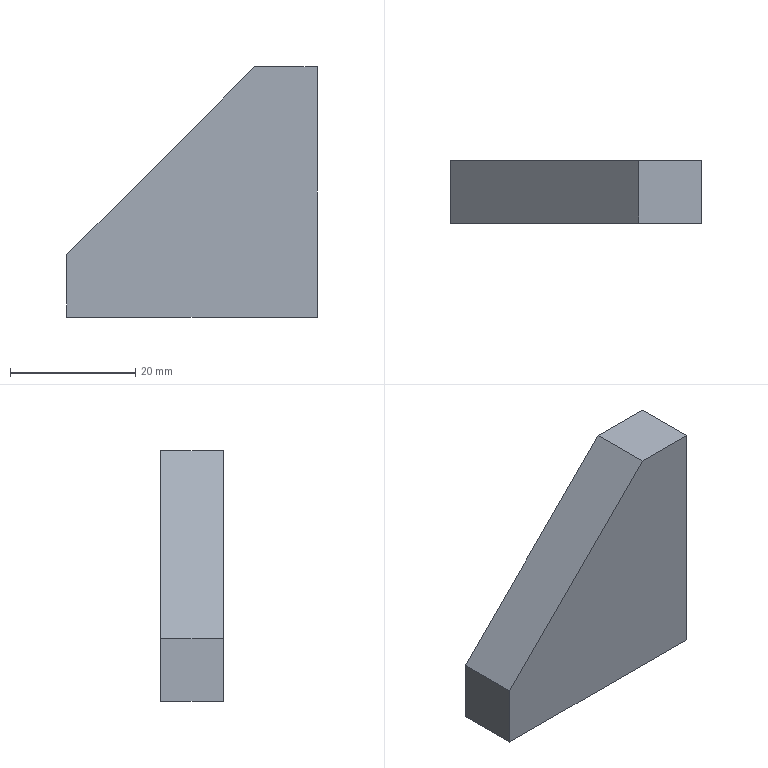Part | STEP file | Camera bracket reinforcement plate | 1 solid | 27 faces | box 40 x 10 x 40 mm | volume 11008 mm3 | cylinder 12 | cone 8 | plane 7 | commonest cylinder face diameters 3.3 x12